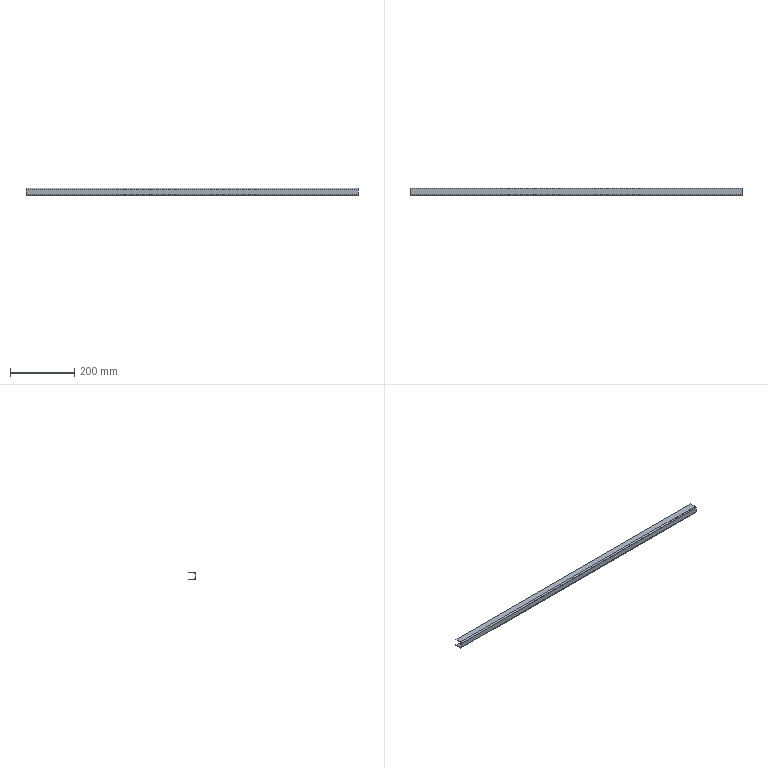Part | NX | features solid 2 | 1 solid | 14 faces | box 1030 x 23 x 23 mm | volume 128595 mm3 | plane 10 | cylinder 4 | commonest cylinder face diameters 4 x2 8 x2
STEP:
#1=CARTESIAN_POINT('',(1160.,-671.,567.));
#2=VERTEX_POINT('',#1);
#3=CARTESIAN_POINT('',(1160.,-652.,567.));
#4=VERTEX_POINT('',#3);
#5=CARTESIAN_POINT('',(1160.,-675.,567.));
#6=DIRECTION('',(0.,1.,0.));
#7=VECTOR('',#6,1000.);
#8=LINE('',#5,#7);
#9=EDGE_CURVE('',#2,#4,#8,.T.);
#10=ORIENTED_EDGE('',*,*,#9,.T.);
#11=CARTESIAN_POINT('',(2190.,-652.,567.));
#12=VERTEX_POINT('',#11);
#13=CARTESIAN_POINT('',(2190.,-652.,567.));
#14=DIRECTION('',(-1.,0.,0.));
#15=VECTOR('',#14,1000.);
#16=LINE('',#13,#15);
#17=EDGE_CURVE('',#12,#4,#16,.T.);
#18=ORIENTED_EDGE('',*,*,#17,.F.);
#19=CARTESIAN_POINT('',(2190.,-671.,567.));
#20=VERTEX_POINT('',#19);
#21=CARTESIAN_POINT('',(2190.,-675.,567.));
#22=DIRECTION('',(0.,1.,0.));
#23=VECTOR('',#22,1000.);
#24=LINE('',#21,#23);
#25=EDGE_CURVE('',#20,#12,#24,.T.);
#26=ORIENTED_EDGE('',*,*,#25,.F.);
#27=CARTESIAN_POINT('',(2190.,-671.,567.));
#28=DIRECTION('',(-1.,0.,0.));
#29=VECTOR('',#28,1000.);
#30=LINE('',#27,#29);
#31=EDGE_CURVE('',#20,#2,#30,.T.);
#32=ORIENTED_EDGE('',*,*,#31,.T.);
#33=EDGE_LOOP('',(#10,#18,#26,#32));
#34=FACE_BOUND('',#33,.T.);
#35=CARTESIAN_POINT('',(2190.,-675.,567.));
#36=DIRECTION('',(0.,0.,1.));
#37=DIRECTION('',(1.,0.,0.));
#38=AXIS2_PLACEMENT_3D('',#35,#36,#37);
#39=PLANE('',#38);
#40=ADVANCED_FACE('',(#34),#39,.F.);
#41=CARTESIAN_POINT('',(1160.,-675.,571.));
#42=VERTEX_POINT('',#41);
#43=CARTESIAN_POINT('',(1160.,-671.,571.));
#44=DIRECTION('',(1.,0.,0.));
#45=DIRECTION('',(0.,-1.,0.));
#46=AXIS2_PLACEMENT_3D('',#43,#44,#45);
#47=CIRCLE('',#46,4.);
#48=EDGE_CURVE('',#42,#2,#47,.T.);
#49=ORIENTED_EDGE('',*,*,#48,.T.);
#50=ORIENTED_EDGE('',*,*,#31,.F.);
#51=CARTESIAN_POINT('',(2190.,-675.,571.));
#52=VERTEX_POINT('',#51);
#53=CARTESIAN_POINT('',(2190.,-671.,571.));
#54=DIRECTION('',(1.,0.,0.));
#55=DIRECTION('',(0.,-1.,0.));
#56=AXIS2_PLACEMENT_3D('',#53,#54,#55);
#57=CIRCLE('',#56,4.);
#58=EDGE_CURVE('',#52,#20,#57,.T.);
#59=ORIENTED_EDGE('',*,*,#58,.F.);
#60=CARTESIAN_POINT('',(2190.,-675.,571.));
#61=DIRECTION('',(-1.,0.,0.));
#62=VECTOR('',#61,1000.);
#63=LINE('',#60,#62);
#64=EDGE_CURVE('',#52,#42,#63,.T.);
#65=ORIENTED_EDGE('',*,*,#64,.T.);
#66=EDGE_LOOP('',(#49,#50,#59,#65));
#67=FACE_BOUND('',#66,.T.);
#68=CARTESIAN_POINT('',(2190.,-671.,571.));
#69=DIRECTION('',(-1.,0.,0.));
#70=DIRECTION('',(0.,-1.,0.));
#71=AXIS2_PLACEMENT_3D('',#68,#69,#70);
#72=CYLINDRICAL_SURFACE('',#71,4.);
#73=ADVANCED_FACE('',(#67),#72,.T.);
#74=CARTESIAN_POINT('',(1160.,-675.,586.));
#75=VERTEX_POINT('',#74);
#76=CARTESIAN_POINT('',(1160.,-675.,590.));
#77=DIRECTION('',(0.,0.,-1.));
#78=VECTOR('',#77,1000.);
#79=LINE('',#76,#78);
#80=EDGE_CURVE('',#75,#42,#79,.T.);
#81=ORIENTED_EDGE('',*,*,#80,.T.);
#82=ORIENTED_EDGE('',*,*,#64,.F.);
#83=CARTESIAN_POINT('',(2190.,-675.,586.));
#84=VERTEX_POINT('',#83);
#85=CARTESIAN_POINT('',(2190.,-675.,590.));
#86=DIRECTION('',(0.,0.,-1.));
#87=VECTOR('',#86,1000.);
#88=LINE('',#85,#87);
#89=EDGE_CURVE('',#84,#52,#88,.T.);
#90=ORIENTED_EDGE('',*,*,#89,.F.);
#91=CARTESIAN_POINT('',(2190.,-675.,586.));
#92=DIRECTION('',(-1.,0.,0.));
#93=VECTOR('',#92,1000.);
#94=LINE('',#91,#93);
#95=EDGE_CURVE('',#84,#75,#94,.T.);
#96=ORIENTED_EDGE('',*,*,#95,.T.);
#97=EDGE_LOOP('',(#81,#82,#90,#96));
#98=FACE_BOUND('',#97,.T.);
#99=CARTESIAN_POINT('',(2190.,-675.,590.));
#100=DIRECTION('',(0.,1.,0.));
#101=DIRECTION('',(0.,0.,-1.));
#102=AXIS2_PLACEMENT_3D('',#99,#100,#101);
#103=PLANE('',#102);
#104=ADVANCED_FACE('',(#98),#103,.F.);
#105=CARTESIAN_POINT('',(1160.,-671.,590.));
#106=VERTEX_POINT('',#105);
#107=CARTESIAN_POINT('',(1160.,-671.,586.));
#108=DIRECTION('',(1.,0.,0.));
#109=DIRECTION('',(0.,-1.,0.));
#110=AXIS2_PLACEMENT_3D('',#107,#108,#109);
#111=CIRCLE('',#110,4.);
#112=EDGE_CURVE('',#106,#75,#111,.T.);
#113=ORIENTED_EDGE('',*,*,#112,.T.);
#114=ORIENTED_EDGE('',*,*,#95,.F.);
#115=CARTESIAN_POINT('',(2190.,-671.,590.));
#116=VERTEX_POINT('',#115);
#117=CARTESIAN_POINT('',(2190.,-671.,586.));
#118=DIRECTION('',(1.,0.,0.));
#119=DIRECTION('',(0.,-1.,0.));
#120=AXIS2_PLACEMENT_3D('',#117,#118,#119);
#121=CIRCLE('',#120,4.);
#122=EDGE_CURVE('',#116,#84,#121,.T.);
#123=ORIENTED_EDGE('',*,*,#122,.F.);
#124=CARTESIAN_POINT('',(2190.,-671.,590.));
#125=DIRECTION('',(-1.,0.,0.));
#126=VECTOR('',#125,1000.);
#127=LINE('',#124,#126);
#128=EDGE_CURVE('',#116,#106,#127,.T.);
#129=ORIENTED_EDGE('',*,*,#128,.T.);
#130=EDGE_LOOP('',(#113,#114,#123,#129));
#131=FACE_BOUND('',#130,.T.);
#132=CARTESIAN_POINT('',(2190.,-671.,586.));
#133=DIRECTION('',(-1.,0.,0.));
#134=DIRECTION('',(0.,-1.,0.));
#135=AXIS2_PLACEMENT_3D('',#132,#133,#134);
#136=CYLINDRICAL_SURFACE('',#135,4.);
#137=ADVANCED_FACE('',(#131),#136,.T.);
#138=CARTESIAN_POINT('',(1160.,-652.,590.));
#139=VERTEX_POINT('',#138);
#140=CARTESIAN_POINT('',(1160.,-652.,590.));
#141=DIRECTION('',(0.,-1.,0.));
#142=VECTOR('',#141,1000.);
#143=LINE('',#140,#142);
#144=EDGE_CURVE('',#139,#106,#143,.T.);
#145=ORIENTED_EDGE('',*,*,#144,.T.);
#146=ORIENTED_EDGE('',*,*,#128,.F.);
#147=CARTESIAN_POINT('',(2190.,-652.,590.));
#148=VERTEX_POINT('',#147);
#149=CARTESIAN_POINT('',(2190.,-652.,590.));
#150=DIRECTION('',(0.,-1.,0.));
#151=VECTOR('',#150,1000.);
#152=LINE('',#149,#151);
#153=EDGE_CURVE('',#148,#116,#152,.T.);
#154=ORIENTED_EDGE('',*,*,#153,.F.);
#155=CARTESIAN_POINT('',(2190.,-652.,590.));
#156=DIRECTION('',(-1.,0.,0.));
#157=VECTOR('',#156,1000.);
#158=LINE('',#155,#157);
#159=EDGE_CURVE('',#148,#139,#158,.T.);
#160=ORIENTED_EDGE('',*,*,#159,.T.);
#161=EDGE_LOOP('',(#145,#146,#154,#160));
#162=FACE_BOUND('',#161,.T.);
#163=CARTESIAN_POINT('',(2190.,-652.,590.));
#164=DIRECTION('',(0.,0.,-1.));
#165=DIRECTION('',(0.,-1.,0.));
#166=AXIS2_PLACEMENT_3D('',#163,#164,#165);
#167=PLANE('',#166);
#168=ADVANCED_FACE('',(#162),#167,.F.);
#169=CARTESIAN_POINT('',(1160.,-671.,569.));
#170=VERTEX_POINT('',#169);
#171=CARTESIAN_POINT('',(1160.,-652.,569.));
#172=VERTEX_POINT('',#171);
#173=CARTESIAN_POINT('',(1160.,-675.,569.));
#174=DIRECTION('',(0.,1.,0.));
#175=VECTOR('',#174,1000.);
#176=LINE('',#173,#175);
#177=EDGE_CURVE('',#170,#172,#176,.T.);
#178=ORIENTED_EDGE('',*,*,#177,.F.);
#179=CARTESIAN_POINT('',(2190.,-671.,569.));
#180=VERTEX_POINT('',#179);
#181=CARTESIAN_POINT('',(2190.,-671.,569.));
#182=DIRECTION('',(-1.,0.,0.));
#183=VECTOR('',#182,1000.);
#184=LINE('',#181,#183);
#185=EDGE_CURVE('',#180,#170,#184,.T.);
#186=ORIENTED_EDGE('',*,*,#185,.F.);
#187=CARTESIAN_POINT('',(2190.,-652.,569.));
#188=VERTEX_POINT('',#187);
#189=CARTESIAN_POINT('',(2190.,-675.,569.));
#190=DIRECTION('',(0.,1.,0.));
#191=VECTOR('',#190,1000.);
#192=LINE('',#189,#191);
#193=EDGE_CURVE('',#180,#188,#192,.T.);
#194=ORIENTED_EDGE('',*,*,#193,.T.);
#195=CARTESIAN_POINT('',(2190.,-652.,569.));
#196=DIRECTION('',(-1.,0.,0.));
#197=VECTOR('',#196,1000.);
#198=LINE('',#195,#197);
#199=EDGE_CURVE('',#188,#172,#198,.T.);
#200=ORIENTED_EDGE('',*,*,#199,.T.);
#201=EDGE_LOOP('',(#178,#186,#194,#200));
#202=FACE_BOUND('',#201,.T.);
#203=CARTESIAN_POINT('',(2190.,-675.,569.));
#204=DIRECTION('',(0.,0.,1.));
#205=DIRECTION('',(1.,0.,0.));
#206=AXIS2_PLACEMENT_3D('',#203,#204,#205);
#207=PLANE('',#206);
#208=ADVANCED_FACE('',(#202),#207,.T.);
#209=CARTESIAN_POINT('',(1160.,-673.,571.));
#210=VERTEX_POINT('',#209);
#211=CARTESIAN_POINT('',(1160.,-671.,571.));
#212=DIRECTION('',(1.,0.,0.));
#213=DIRECTION('',(0.,-1.,0.));
#214=AXIS2_PLACEMENT_3D('',#211,#212,#213);
#215=CIRCLE('',#214,2.);
#216=EDGE_CURVE('',#210,#170,#215,.T.);
#217=ORIENTED_EDGE('',*,*,#216,.F.);
#218=CARTESIAN_POINT('',(2190.,-673.,571.));
#219=VERTEX_POINT('',#218);
#220=CARTESIAN_POINT('',(2190.,-673.,571.));
#221=DIRECTION('',(-1.,0.,0.));
#222=VECTOR('',#221,1000.);
#223=LINE('',#220,#222);
#224=EDGE_CURVE('',#219,#210,#223,.T.);
#225=ORIENTED_EDGE('',*,*,#224,.F.);
#226=CARTESIAN_POINT('',(2190.,-671.,571.));
#227=DIRECTION('',(1.,0.,0.));
#228=DIRECTION('',(0.,-1.,0.));
#229=AXIS2_PLACEMENT_3D('',#226,#227,#228);
#230=CIRCLE('',#229,2.);
#231=EDGE_CURVE('',#219,#180,#230,.T.);
#232=ORIENTED_EDGE('',*,*,#231,.T.);
#233=ORIENTED_EDGE('',*,*,#185,.T.);
#234=EDGE_LOOP('',(#217,#225,#232,#233));
#235=FACE_BOUND('',#234,.T.);
#236=CARTESIAN_POINT('',(2190.,-671.,571.));
#237=DIRECTION('',(-1.,0.,0.));
#238=DIRECTION('',(0.,-1.,0.));
#239=AXIS2_PLACEMENT_3D('',#236,#237,#238);
#240=CYLINDRICAL_SURFACE('',#239,2.);
#241=ADVANCED_FACE('',(#235),#240,.F.);
#242=CARTESIAN_POINT('',(1160.,-673.,586.));
#243=VERTEX_POINT('',#242);
#244=CARTESIAN_POINT('',(1160.,-673.,590.));
#245=DIRECTION('',(0.,0.,-1.));
#246=VECTOR('',#245,1000.);
#247=LINE('',#244,#246);
#248=EDGE_CURVE('',#243,#210,#247,.T.);
#249=ORIENTED_EDGE('',*,*,#248,.F.);
#250=CARTESIAN_POINT('',(2190.,-673.,586.));
#251=VERTEX_POINT('',#250);
#252=CARTESIAN_POINT('',(2190.,-673.,586.));
#253=DIRECTION('',(-1.,0.,0.));
#254=VECTOR('',#253,1000.);
#255=LINE('',#252,#254);
#256=EDGE_CURVE('',#251,#243,#255,.T.);
#257=ORIENTED_EDGE('',*,*,#256,.F.);
#258=CARTESIAN_POINT('',(2190.,-673.,590.));
#259=DIRECTION('',(0.,0.,-1.));
#260=VECTOR('',#259,1000.);
#261=LINE('',#258,#260);
#262=EDGE_CURVE('',#251,#219,#261,.T.);
#263=ORIENTED_EDGE('',*,*,#262,.T.);
#264=ORIENTED_EDGE('',*,*,#224,.T.);
#265=EDGE_LOOP('',(#249,#257,#263,#264));
#266=FACE_BOUND('',#265,.T.);
#267=CARTESIAN_POINT('',(2190.,-673.,590.));
#268=DIRECTION('',(0.,1.,0.));
#269=DIRECTION('',(0.,0.,-1.));
#270=AXIS2_PLACEMENT_3D('',#267,#268,#269);
#271=PLANE('',#270);
#272=ADVANCED_FACE('',(#266),#271,.T.);
#273=CARTESIAN_POINT('',(1160.,-671.,588.));
#274=VERTEX_POINT('',#273);
#275=CARTESIAN_POINT('',(1160.,-671.,586.));
#276=DIRECTION('',(1.,0.,0.));
#277=DIRECTION('',(0.,-1.,0.));
#278=AXIS2_PLACEMENT_3D('',#275,#276,#277);
#279=CIRCLE('',#278,2.);
#280=EDGE_CURVE('',#274,#243,#279,.T.);
#281=ORIENTED_EDGE('',*,*,#280,.F.);
#282=CARTESIAN_POINT('',(2190.,-671.,588.));
#283=VERTEX_POINT('',#282);
#284=CARTESIAN_POINT('',(2190.,-671.,588.));
#285=DIRECTION('',(-1.,0.,0.));
#286=VECTOR('',#285,1000.);
#287=LINE('',#284,#286);
#288=EDGE_CURVE('',#283,#274,#287,.T.);
#289=ORIENTED_EDGE('',*,*,#288,.F.);
#290=CARTESIAN_POINT('',(2190.,-671.,586.));
#291=DIRECTION('',(1.,0.,0.));
#292=DIRECTION('',(0.,-1.,0.));
#293=AXIS2_PLACEMENT_3D('',#290,#291,#292);
#294=CIRCLE('',#293,2.);
#295=EDGE_CURVE('',#283,#251,#294,.T.);
#296=ORIENTED_EDGE('',*,*,#295,.T.);
#297=ORIENTED_EDGE('',*,*,#256,.T.);
#298=EDGE_LOOP('',(#281,#289,#296,#297));
#299=FACE_BOUND('',#298,.T.);
#300=CARTESIAN_POINT('',(2190.,-671.,586.));
#301=DIRECTION('',(-1.,0.,0.));
#302=DIRECTION('',(0.,-1.,0.));
#303=AXIS2_PLACEMENT_3D('',#300,#301,#302);
#304=CYLINDRICAL_SURFACE('',#303,2.);
#305=ADVANCED_FACE('',(#299),#304,.F.);
#306=CARTESIAN_POINT('',(1160.,-652.,588.));
#307=VERTEX_POINT('',#306);
#308=CARTESIAN_POINT('',(1160.,-652.,588.));
#309=DIRECTION('',(0.,-1.,0.));
#310=VECTOR('',#309,1000.);
#311=LINE('',#308,#310);
#312=EDGE_CURVE('',#307,#274,#311,.T.);
#313=ORIENTED_EDGE('',*,*,#312,.F.);
#314=CARTESIAN_POINT('',(2190.,-652.,588.));
#315=VERTEX_POINT('',#314);
#316=CARTESIAN_POINT('',(2190.,-652.,588.));
#317=DIRECTION('',(-1.,0.,0.));
#318=VECTOR('',#317,1000.);
#319=LINE('',#316,#318);
#320=EDGE_CURVE('',#315,#307,#319,.T.);
#321=ORIENTED_EDGE('',*,*,#320,.F.);
#322=CARTESIAN_POINT('',(2190.,-652.,588.));
#323=DIRECTION('',(0.,-1.,0.));
#324=VECTOR('',#323,1000.);
#325=LINE('',#322,#324);
#326=EDGE_CURVE('',#315,#283,#325,.T.);
#327=ORIENTED_EDGE('',*,*,#326,.T.);
#328=ORIENTED_EDGE('',*,*,#288,.T.);
#329=EDGE_LOOP('',(#313,#321,#327,#328));
#330=FACE_BOUND('',#329,.T.);
#331=CARTESIAN_POINT('',(2190.,-652.,588.));
#332=DIRECTION('',(0.,0.,-1.));
#333=DIRECTION('',(0.,-1.,0.));
#334=AXIS2_PLACEMENT_3D('',#331,#332,#333);
#335=PLANE('',#334);
#336=ADVANCED_FACE('',(#330),#335,.T.);
#337=ORIENTED_EDGE('',*,*,#159,.F.);
#338=CARTESIAN_POINT('',(2190.,-652.,590.));
#339=DIRECTION('',(0.,0.,-1.));
#340=VECTOR('',#339,1000.);
#341=LINE('',#338,#340);
#342=EDGE_CURVE('',#148,#315,#341,.T.);
#343=ORIENTED_EDGE('',*,*,#342,.T.);
#344=ORIENTED_EDGE('',*,*,#320,.T.);
#345=CARTESIAN_POINT('',(1160.,-652.,590.));
#346=DIRECTION('',(0.,0.,-1.));
#347=VECTOR('',#346,1000.);
#348=LINE('',#345,#347);
#349=EDGE_CURVE('',#139,#307,#348,.T.);
#350=ORIENTED_EDGE('',*,*,#349,.F.);
#351=EDGE_LOOP('',(#337,#343,#344,#350));
#352=FACE_BOUND('',#351,.T.);
#353=CARTESIAN_POINT('',(2190.,-652.,590.));
#354=DIRECTION('',(0.,-1.,0.));
#355=DIRECTION('',(-1.,0.,0.));
#356=AXIS2_PLACEMENT_3D('',#353,#354,#355);
#357=PLANE('',#356);
#358=ADVANCED_FACE('',(#352),#357,.F.);
#359=ORIENTED_EDGE('',*,*,#312,.T.);
#360=ORIENTED_EDGE('',*,*,#280,.T.);
#361=ORIENTED_EDGE('',*,*,#248,.T.);
#362=ORIENTED_EDGE('',*,*,#216,.T.);
#363=ORIENTED_EDGE('',*,*,#177,.T.);
#364=CARTESIAN_POINT('',(1160.,-652.,567.));
#365=DIRECTION('',(0.,0.,1.));
#366=VECTOR('',#365,1000.);
#367=LINE('',#364,#366);
#368=EDGE_CURVE('',#4,#172,#367,.T.);
#369=ORIENTED_EDGE('',*,*,#368,.F.);
#370=ORIENTED_EDGE('',*,*,#9,.F.);
#371=ORIENTED_EDGE('',*,*,#48,.F.);
#372=ORIENTED_EDGE('',*,*,#80,.F.);
#373=ORIENTED_EDGE('',*,*,#112,.F.);
#374=ORIENTED_EDGE('',*,*,#144,.F.);
#375=ORIENTED_EDGE('',*,*,#349,.T.);
#376=EDGE_LOOP('',(#359,#360,#361,#362,#363,#369,#370,#371,#372,#373,#374,#375));
#377=FACE_BOUND('',#376,.T.);
#378=CARTESIAN_POINT('',(1160.,-652.,590.));
#379=DIRECTION('',(1.,0.,0.));
#380=DIRECTION('',(0.,0.,1.));
#381=AXIS2_PLACEMENT_3D('',#378,#379,#380);
#382=PLANE('',#381);
#383=ADVANCED_FACE('',(#377),#382,.F.);
#384=CARTESIAN_POINT('',(2190.,-652.,567.));
#385=DIRECTION('',(0.,0.,1.));
#386=VECTOR('',#385,1000.);
#387=LINE('',#384,#386);
#388=EDGE_CURVE('',#12,#188,#387,.T.);
#389=ORIENTED_EDGE('',*,*,#388,.F.);
#390=ORIENTED_EDGE('',*,*,#17,.T.);
#391=ORIENTED_EDGE('',*,*,#368,.T.);
#392=ORIENTED_EDGE('',*,*,#199,.F.);
#393=EDGE_LOOP('',(#389,#390,#391,#392));
#394=FACE_BOUND('',#393,.T.);
#395=CARTESIAN_POINT('',(2190.,-652.,567.));
#396=DIRECTION('',(0.,1.,0.));
#397=DIRECTION('',(0.,0.,-1.));
#398=AXIS2_PLACEMENT_3D('',#395,#396,#397);
#399=PLANE('',#398);
#400=ADVANCED_FACE('',(#394),#399,.T.);
#401=ORIENTED_EDGE('',*,*,#193,.F.);
#402=ORIENTED_EDGE('',*,*,#231,.F.);
#403=ORIENTED_EDGE('',*,*,#262,.F.);
#404=ORIENTED_EDGE('',*,*,#295,.F.);
#405=ORIENTED_EDGE('',*,*,#326,.F.);
#406=ORIENTED_EDGE('',*,*,#342,.F.);
#407=ORIENTED_EDGE('',*,*,#153,.T.);
#408=ORIENTED_EDGE('',*,*,#122,.T.);
#409=ORIENTED_EDGE('',*,*,#89,.T.);
#410=ORIENTED_EDGE('',*,*,#58,.T.);
#411=ORIENTED_EDGE('',*,*,#25,.T.);
#412=ORIENTED_EDGE('',*,*,#388,.T.);
#413=EDGE_LOOP('',(#401,#402,#403,#404,#405,#406,#407,#408,#409,#410,#411,#412));
#414=FACE_BOUND('',#413,.T.);
#415=CARTESIAN_POINT('',(2190.,-675.,567.));
#416=DIRECTION('',(1.,0.,0.));
#417=DIRECTION('',(0.,0.,1.));
#418=AXIS2_PLACEMENT_3D('',#415,#416,#417);
#419=PLANE('',#418);
#420=ADVANCED_FACE('',(#414),#419,.T.);
#421=CLOSED_SHELL('',(#40,#73,#104,#137,#168,#208,#241,#272,#305,#336,#358,#383,#400,#420));
#422=MANIFOLD_SOLID_BREP('',#421);
#423=(LENGTH_UNIT()NAMED_UNIT(*)SI_UNIT(.MILLI.,.METRE.));
#424=UNCERTAINTY_MEASURE_WITH_UNIT(LENGTH_MEASURE(0.00001),#423,'','');
#425=(NAMED_UNIT(*)PLANE_ANGLE_UNIT()SI_UNIT($,.RADIAN.));
#426=(NAMED_UNIT(*)SI_UNIT($,.STERADIAN.)SOLID_ANGLE_UNIT());
#427=(GEOMETRIC_REPRESENTATION_CONTEXT(3)GLOBAL_UNCERTAINTY_ASSIGNED_CONTEXT((#424))GLOBAL_UNIT_ASSIGNED_CONTEXT((#423,#425,#426))REPRESENTATION_CONTEXT('',''));
#428=ADVANCED_BREP_SHAPE_REPRESENTATION('',(#422),#427);